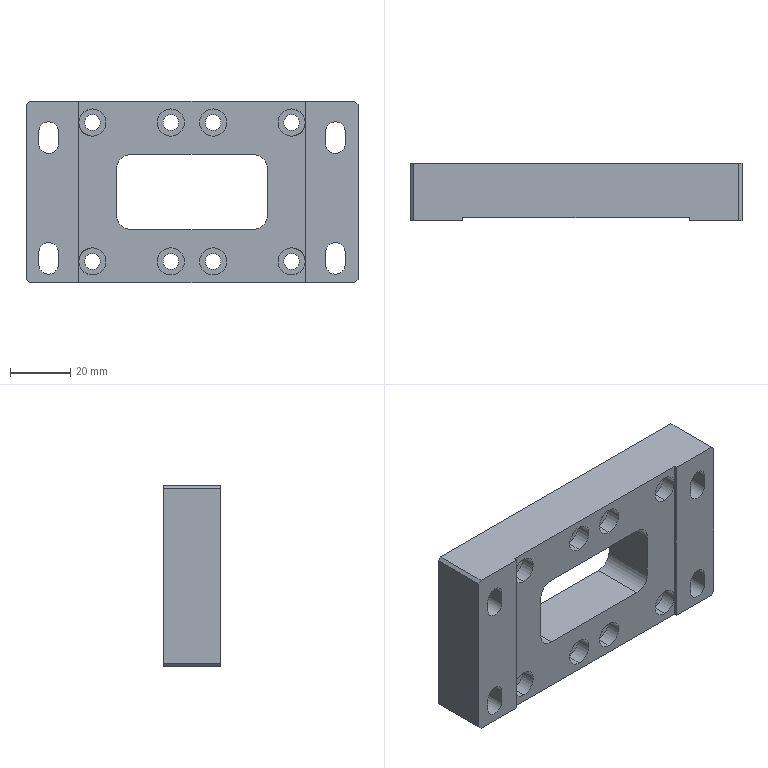Part | STEP file | 1 solid | 106 faces | box 110 x 19 x 60 mm | volume 87261 mm3 | cylinder 60 | plane 46 | commonest cylinder face diameters 5.2 x16 9 x16 6.5 x12 11 x12 10 x4